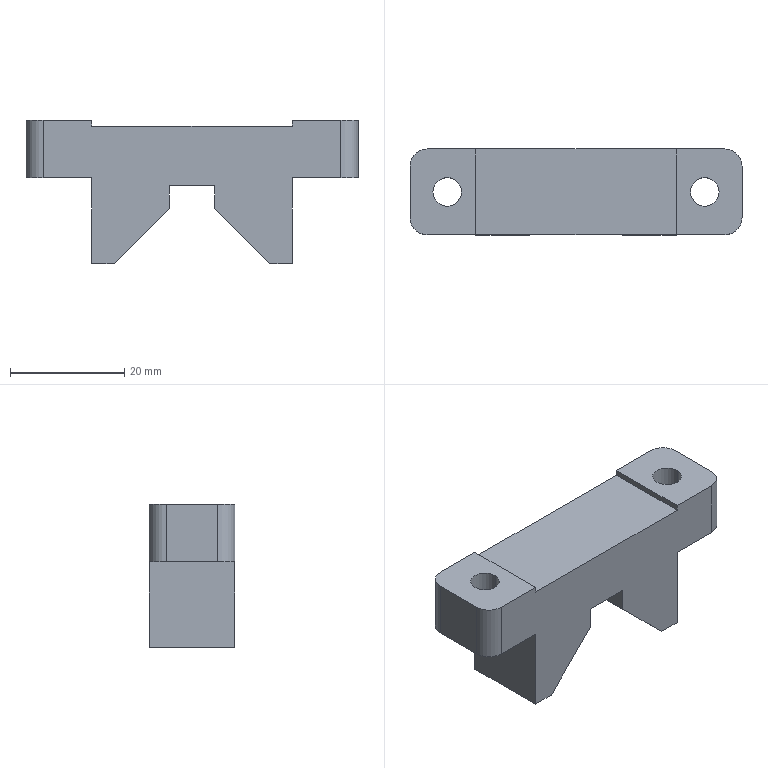Part | SolidWorks | features ICE 2, BaseBody 1, Fillet 1 | 1 solid | 28 faces | box 58 x 15 x 25 mm | volume 12562 mm3 | plane 20 | cylinder 8 | commonest cylinder face diameters 5 x4 6 x4
STEP:
#1=CARTESIAN_POINT('',(60.,7.5,-10.));
#2=VERTEX_POINT('',#1);
#3=CARTESIAN_POINT('',(65.,7.5,-10.));
#4=VERTEX_POINT('',#3);
#5=CARTESIAN_POINT('',(62.5,7.5,-10.));
#6=DIRECTION('',(0.,0.,1.));
#7=DIRECTION('',(1.,0.,0.));
#8=AXIS2_PLACEMENT_3D('',#5,#6,#7);
#9=CIRCLE('',#8,2.5);
#10=EDGE_CURVE('',#2,#4,#9,.T.);
#11=ORIENTED_EDGE('',*,*,#10,.F.);
#12=CARTESIAN_POINT('',(60.,7.5,0.));
#13=VERTEX_POINT('',#12);
#14=CARTESIAN_POINT('',(60.,7.5,-10.));
#15=DIRECTION('',(0.,0.,1.));
#16=VECTOR('',#15,1000.);
#17=LINE('',#14,#16);
#18=EDGE_CURVE('',#2,#13,#17,.T.);
#19=ORIENTED_EDGE('',*,*,#18,.T.);
#20=CARTESIAN_POINT('',(65.,7.5,0.));
#21=VERTEX_POINT('',#20);
#22=CARTESIAN_POINT('',(62.5,7.5,0.));
#23=DIRECTION('',(0.,0.,1.));
#24=DIRECTION('',(1.,0.,0.));
#25=AXIS2_PLACEMENT_3D('',#22,#23,#24);
#26=CIRCLE('',#25,2.5);
#27=EDGE_CURVE('',#13,#21,#26,.T.);
#28=ORIENTED_EDGE('',*,*,#27,.T.);
#29=CARTESIAN_POINT('',(65.,7.5,-10.));
#30=DIRECTION('',(0.,0.,1.));
#31=VECTOR('',#30,1000.);
#32=LINE('',#29,#31);
#33=EDGE_CURVE('',#4,#21,#32,.T.);
#34=ORIENTED_EDGE('',*,*,#33,.F.);
#35=EDGE_LOOP('',(#11,#19,#28,#34));
#36=FACE_OUTER_BOUND('',#35,.T.);
#37=CARTESIAN_POINT('',(62.5,7.5,-10.));
#38=DIRECTION('',(0.,0.,1.));
#39=DIRECTION('',(1.,0.,0.));
#40=AXIS2_PLACEMENT_3D('',#37,#38,#39);
#41=CYLINDRICAL_SURFACE('',#40,2.5);
#42=ADVANCED_FACE('',(#36),#41,.F.);
#43=CARTESIAN_POINT('',(20.,7.5,-10.));
#44=VERTEX_POINT('',#43);
#45=CARTESIAN_POINT('',(15.,7.5,-10.));
#46=VERTEX_POINT('',#45);
#47=CARTESIAN_POINT('',(17.5,7.5,-10.));
#48=DIRECTION('',(0.,0.,-1.));
#49=DIRECTION('',(1.,0.,0.));
#50=AXIS2_PLACEMENT_3D('',#47,#48,#49);
#51=CIRCLE('',#50,2.5);
#52=EDGE_CURVE('',#44,#46,#51,.T.);
#53=ORIENTED_EDGE('',*,*,#52,.T.);
#54=CARTESIAN_POINT('',(15.,7.5,0.));
#55=VERTEX_POINT('',#54);
#56=CARTESIAN_POINT('',(15.,7.5,-10.));
#57=DIRECTION('',(0.,0.,1.));
#58=VECTOR('',#57,1000.);
#59=LINE('',#56,#58);
#60=EDGE_CURVE('',#46,#55,#59,.T.);
#61=ORIENTED_EDGE('',*,*,#60,.T.);
#62=CARTESIAN_POINT('',(20.,7.5,0.));
#63=VERTEX_POINT('',#62);
#64=CARTESIAN_POINT('',(17.5,7.5,0.));
#65=DIRECTION('',(0.,0.,1.));
#66=DIRECTION('',(1.,0.,0.));
#67=AXIS2_PLACEMENT_3D('',#64,#65,#66);
#68=CIRCLE('',#67,2.5);
#69=EDGE_CURVE('',#55,#63,#68,.T.);
#70=ORIENTED_EDGE('',*,*,#69,.T.);
#71=CARTESIAN_POINT('',(20.,7.5,-10.));
#72=DIRECTION('',(0.,0.,1.));
#73=VECTOR('',#72,1000.);
#74=LINE('',#71,#73);
#75=EDGE_CURVE('',#44,#63,#74,.T.);
#76=ORIENTED_EDGE('',*,*,#75,.F.);
#77=EDGE_LOOP('',(#53,#61,#70,#76));
#78=FACE_OUTER_BOUND('',#77,.T.);
#79=CARTESIAN_POINT('',(17.5,7.5,-10.));
#80=DIRECTION('',(0.,0.,1.));
#81=DIRECTION('',(1.,0.,0.));
#82=AXIS2_PLACEMENT_3D('',#79,#80,#81);
#83=CYLINDRICAL_SURFACE('',#82,2.5);
#84=ADVANCED_FACE('',(#78),#83,.F.);
#85=CARTESIAN_POINT('',(62.5,7.5,0.));
#86=DIRECTION('',(0.,0.,1.));
#87=DIRECTION('',(1.,0.,0.));
#88=AXIS2_PLACEMENT_3D('',#85,#86,#87);
#89=CIRCLE('',#88,2.5);
#90=EDGE_CURVE('',#21,#13,#89,.T.);
#91=ORIENTED_EDGE('',*,*,#90,.F.);
#92=ORIENTED_EDGE('',*,*,#27,.F.);
#93=EDGE_LOOP('',(#91,#92));
#94=FACE_BOUND('',#93,.T.);
#95=CARTESIAN_POINT('',(57.5,15.,0.));
#96=VERTEX_POINT('',#95);
#97=CARTESIAN_POINT('',(66.,15.,0.));
#98=VERTEX_POINT('',#97);
#99=CARTESIAN_POINT('',(0.,15.,0.));
#100=DIRECTION('',(1.,0.,0.));
#101=VECTOR('',#100,1000.);
#102=LINE('',#99,#101);
#103=EDGE_CURVE('',#96,#98,#102,.T.);
#104=ORIENTED_EDGE('',*,*,#103,.F.);
#105=CARTESIAN_POINT('',(57.5,0.,0.));
#106=VERTEX_POINT('',#105);
#107=CARTESIAN_POINT('',(57.5,15.,0.));
#108=DIRECTION('',(0.,-1.,0.));
#109=VECTOR('',#108,1000.);
#110=LINE('',#107,#109);
#111=EDGE_CURVE('',#96,#106,#110,.T.);
#112=ORIENTED_EDGE('',*,*,#111,.T.);
#113=CARTESIAN_POINT('',(66.,0.,0.));
#114=VERTEX_POINT('',#113);
#115=CARTESIAN_POINT('',(0.,0.,0.));
#116=DIRECTION('',(-1.,0.,0.));
#117=VECTOR('',#116,1000.);
#118=LINE('',#115,#117);
#119=EDGE_CURVE('',#114,#106,#118,.T.);
#120=ORIENTED_EDGE('',*,*,#119,.F.);
#121=CARTESIAN_POINT('',(69.,3.,0.));
#122=VERTEX_POINT('',#121);
#123=CARTESIAN_POINT('',(66.,3.,0.));
#124=DIRECTION('',(0.,0.,1.));
#125=DIRECTION('',(-1.,0.,0.));
#126=AXIS2_PLACEMENT_3D('',#123,#124,#125);
#127=CIRCLE('',#126,3.);
#128=EDGE_CURVE('',#114,#122,#127,.T.);
#129=ORIENTED_EDGE('',*,*,#128,.T.);
#130=CARTESIAN_POINT('',(69.,12.,0.));
#131=VERTEX_POINT('',#130);
#132=CARTESIAN_POINT('',(69.,15.,0.));
#133=DIRECTION('',(0.,1.,0.));
#134=VECTOR('',#133,1000.);
#135=LINE('',#132,#134);
#136=EDGE_CURVE('',#122,#131,#135,.T.);
#137=ORIENTED_EDGE('',*,*,#136,.T.);
#138=CARTESIAN_POINT('',(66.,12.,0.));
#139=DIRECTION('',(0.,0.,1.));
#140=DIRECTION('',(-1.,0.,0.));
#141=AXIS2_PLACEMENT_3D('',#138,#139,#140);
#142=CIRCLE('',#141,3.);
#143=EDGE_CURVE('',#131,#98,#142,.T.);
#144=ORIENTED_EDGE('',*,*,#143,.T.);
#145=EDGE_LOOP('',(#104,#112,#120,#129,#137,#144));
#146=FACE_OUTER_BOUND('',#145,.T.);
#147=CARTESIAN_POINT('',(0.,15.,0.));
#148=DIRECTION('',(0.,0.,-1.));
#149=DIRECTION('',(-1.,0.,0.));
#150=AXIS2_PLACEMENT_3D('',#147,#148,#149);
#151=PLANE('',#150);
#152=ADVANCED_FACE('',(#94,#146),#151,.F.);
#153=CARTESIAN_POINT('',(57.5,15.,-1.));
#154=VERTEX_POINT('',#153);
#155=CARTESIAN_POINT('',(57.5,15.,0.));
#156=DIRECTION('',(0.,0.,1.));
#157=VECTOR('',#156,1000.);
#158=LINE('',#155,#157);
#159=EDGE_CURVE('',#154,#96,#158,.T.);
#160=ORIENTED_EDGE('',*,*,#159,.T.);
#161=ORIENTED_EDGE('',*,*,#103,.T.);
#162=CARTESIAN_POINT('',(66.,15.,-10.));
#163=VERTEX_POINT('',#162);
#164=CARTESIAN_POINT('',(66.,15.,-10.));
#165=DIRECTION('',(0.,0.,-1.));
#166=VECTOR('',#165,1000.);
#167=LINE('',#164,#166);
#168=EDGE_CURVE('',#98,#163,#167,.T.);
#169=ORIENTED_EDGE('',*,*,#168,.T.);
#170=CARTESIAN_POINT('',(57.5,15.,-10.));
#171=VERTEX_POINT('',#170);
#172=CARTESIAN_POINT('',(0.,15.,-10.));
#173=DIRECTION('',(-1.,0.,0.));
#174=VECTOR('',#173,1000.);
#175=LINE('',#172,#174);
#176=EDGE_CURVE('',#163,#171,#175,.T.);
#177=ORIENTED_EDGE('',*,*,#176,.T.);
#178=CARTESIAN_POINT('',(57.5,15.,-25.));
#179=VERTEX_POINT('',#178);
#180=CARTESIAN_POINT('',(57.5,15.,0.));
#181=DIRECTION('',(0.,0.,-1.));
#182=VECTOR('',#181,1000.);
#183=LINE('',#180,#182);
#184=EDGE_CURVE('',#171,#179,#183,.T.);
#185=ORIENTED_EDGE('',*,*,#184,.T.);
#186=CARTESIAN_POINT('',(53.61,15.,-25.));
#187=VERTEX_POINT('',#186);
#188=CARTESIAN_POINT('',(0.,15.,-25.));
#189=DIRECTION('',(-1.,0.,0.));
#190=VECTOR('',#189,1000.);
#191=LINE('',#188,#190);
#192=EDGE_CURVE('',#179,#187,#191,.T.);
#193=ORIENTED_EDGE('',*,*,#192,.T.);
#194=CARTESIAN_POINT('',(44.,15.,-15.39));
#195=VERTEX_POINT('',#194);
#196=CARTESIAN_POINT('',(53.61,15.,-25.));
#197=DIRECTION('',(-0.7071,0.,0.7071));
#198=VECTOR('',#197,1000.);
#199=LINE('',#196,#198);
#200=EDGE_CURVE('',#187,#195,#199,.T.);
#201=ORIENTED_EDGE('',*,*,#200,.T.);
#202=CARTESIAN_POINT('',(44.,15.,-11.39));
#203=VERTEX_POINT('',#202);
#204=CARTESIAN_POINT('',(44.,15.,0.));
#205=DIRECTION('',(0.,0.,1.));
#206=VECTOR('',#205,1000.);
#207=LINE('',#204,#206);
#208=EDGE_CURVE('',#195,#203,#207,.T.);
#209=ORIENTED_EDGE('',*,*,#208,.T.);
#210=CARTESIAN_POINT('',(36.,15.,-11.39));
#211=VERTEX_POINT('',#210);
#212=CARTESIAN_POINT('',(0.,15.,-11.39));
#213=DIRECTION('',(-1.,0.,0.));
#214=VECTOR('',#213,1000.);
#215=LINE('',#212,#214);
#216=EDGE_CURVE('',#203,#211,#215,.T.);
#217=ORIENTED_EDGE('',*,*,#216,.T.);
#218=CARTESIAN_POINT('',(36.,15.,-15.39));
#219=VERTEX_POINT('',#218);
#220=CARTESIAN_POINT('',(36.,15.,0.));
#221=DIRECTION('',(0.,0.,-1.));
#222=VECTOR('',#221,1000.);
#223=LINE('',#220,#222);
#224=EDGE_CURVE('',#211,#219,#223,.T.);
#225=ORIENTED_EDGE('',*,*,#224,.T.);
#226=CARTESIAN_POINT('',(26.39,15.,-25.));
#227=VERTEX_POINT('',#226);
#228=CARTESIAN_POINT('',(36.,15.,-15.39));
#229=DIRECTION('',(-0.7071,0.,-0.7071));
#230=VECTOR('',#229,1000.);
#231=LINE('',#228,#230);
#232=EDGE_CURVE('',#219,#227,#231,.T.);
#233=ORIENTED_EDGE('',*,*,#232,.T.);
#234=CARTESIAN_POINT('',(22.5,15.,-25.));
#235=VERTEX_POINT('',#234);
#236=CARTESIAN_POINT('',(0.,15.,-25.));
#237=DIRECTION('',(-1.,0.,0.));
#238=VECTOR('',#237,1000.);
#239=LINE('',#236,#238);
#240=EDGE_CURVE('',#227,#235,#239,.T.);
#241=ORIENTED_EDGE('',*,*,#240,.T.);
#242=CARTESIAN_POINT('',(22.5,15.,-10.));
#243=VERTEX_POINT('',#242);
#244=CARTESIAN_POINT('',(22.5,15.,0.));
#245=DIRECTION('',(0.,0.,1.));
#246=VECTOR('',#245,1000.);
#247=LINE('',#244,#246);
#248=EDGE_CURVE('',#235,#243,#247,.T.);
#249=ORIENTED_EDGE('',*,*,#248,.T.);
#250=CARTESIAN_POINT('',(14.,15.,-10.));
#251=VERTEX_POINT('',#250);
#252=CARTESIAN_POINT('',(0.,15.,-10.));
#253=DIRECTION('',(-1.,0.,0.));
#254=VECTOR('',#253,1000.);
#255=LINE('',#252,#254);
#256=EDGE_CURVE('',#243,#251,#255,.T.);
#257=ORIENTED_EDGE('',*,*,#256,.T.);
#258=CARTESIAN_POINT('',(14.,15.,0.));
#259=VERTEX_POINT('',#258);
#260=CARTESIAN_POINT('',(14.,15.,0.));
#261=DIRECTION('',(0.,0.,1.));
#262=VECTOR('',#261,1000.);
#263=LINE('',#260,#262);
#264=EDGE_CURVE('',#251,#259,#263,.T.);
#265=ORIENTED_EDGE('',*,*,#264,.T.);
#266=CARTESIAN_POINT('',(22.5,15.,0.));
#267=VERTEX_POINT('',#266);
#268=CARTESIAN_POINT('',(0.,15.,0.));
#269=DIRECTION('',(1.,0.,0.));
#270=VECTOR('',#269,1000.);
#271=LINE('',#268,#270);
#272=EDGE_CURVE('',#259,#267,#271,.T.);
#273=ORIENTED_EDGE('',*,*,#272,.T.);
#274=CARTESIAN_POINT('',(22.5,15.,-1.));
#275=VERTEX_POINT('',#274);
#276=CARTESIAN_POINT('',(22.5,15.,0.));
#277=DIRECTION('',(0.,0.,-1.));
#278=VECTOR('',#277,1000.);
#279=LINE('',#276,#278);
#280=EDGE_CURVE('',#267,#275,#279,.T.);
#281=ORIENTED_EDGE('',*,*,#280,.T.);
#282=CARTESIAN_POINT('',(57.5,15.,-1.));
#283=DIRECTION('',(1.,0.,0.));
#284=VECTOR('',#283,1000.);
#285=LINE('',#282,#284);
#286=EDGE_CURVE('',#275,#154,#285,.T.);
#287=ORIENTED_EDGE('',*,*,#286,.T.);
#288=EDGE_LOOP('',(#160,#161,#169,#177,#185,#193,#201,#209,#217,#225,#233,#241,#249,#257,#265,#273,#281,#287));
#289=FACE_OUTER_BOUND('',#288,.T.);
#290=CARTESIAN_POINT('',(0.,15.,0.));
#291=DIRECTION('',(0.,1.,0.));
#292=DIRECTION('',(0.,0.,1.));
#293=AXIS2_PLACEMENT_3D('',#290,#291,#292);
#294=PLANE('',#293);
#295=ADVANCED_FACE('',(#289),#294,.T.);
#296=CARTESIAN_POINT('',(36.,0.,-11.39));
#297=VERTEX_POINT('',#296);
#298=CARTESIAN_POINT('',(36.,16.5,-11.39));
#299=DIRECTION('',(0.,1.,0.));
#300=VECTOR('',#299,1000.);
#301=LINE('',#298,#300);
#302=EDGE_CURVE('',#297,#211,#301,.T.);
#303=ORIENTED_EDGE('',*,*,#302,.F.);
#304=CARTESIAN_POINT('',(36.,0.,-15.39));
#305=VERTEX_POINT('',#304);
#306=CARTESIAN_POINT('',(36.,0.,-11.39));
#307=DIRECTION('',(0.,0.,1.));
#308=VECTOR('',#307,1000.);
#309=LINE('',#306,#308);
#310=EDGE_CURVE('',#305,#297,#309,.T.);
#311=ORIENTED_EDGE('',*,*,#310,.F.);
#312=CARTESIAN_POINT('',(36.,16.5,-15.39));
#313=DIRECTION('',(0.,-1.,0.));
#314=VECTOR('',#313,1000.);
#315=LINE('',#312,#314);
#316=EDGE_CURVE('',#219,#305,#315,.T.);
#317=ORIENTED_EDGE('',*,*,#316,.F.);
#318=ORIENTED_EDGE('',*,*,#224,.F.);
#319=EDGE_LOOP('',(#303,#311,#317,#318));
#320=FACE_OUTER_BOUND('',#319,.T.);
#321=CARTESIAN_POINT('',(36.,16.5,-11.39));
#322=DIRECTION('',(-1.,0.,0.));
#323=DIRECTION('',(0.,0.,1.));
#324=AXIS2_PLACEMENT_3D('',#321,#322,#323);
#325=PLANE('',#324);
#326=ADVANCED_FACE('',(#320),#325,.F.);
#327=CARTESIAN_POINT('',(44.,0.,-11.39));
#328=VERTEX_POINT('',#327);
#329=CARTESIAN_POINT('',(44.,16.5,-11.39));
#330=DIRECTION('',(0.,1.,0.));
#331=VECTOR('',#330,1000.);
#332=LINE('',#329,#331);
#333=EDGE_CURVE('',#328,#203,#332,.T.);
#334=ORIENTED_EDGE('',*,*,#333,.F.);
#335=CARTESIAN_POINT('',(44.,0.,-11.39));
#336=DIRECTION('',(1.,0.,0.));
#337=VECTOR('',#336,1000.);
#338=LINE('',#335,#337);
#339=EDGE_CURVE('',#297,#328,#338,.T.);
#340=ORIENTED_EDGE('',*,*,#339,.F.);
#341=ORIENTED_EDGE('',*,*,#302,.T.);
#342=ORIENTED_EDGE('',*,*,#216,.F.);
#343=EDGE_LOOP('',(#334,#340,#341,#342));
#344=FACE_OUTER_BOUND('',#343,.T.);
#345=CARTESIAN_POINT('',(44.,16.5,-11.39));
#346=DIRECTION('',(0.,0.,1.));
#347=DIRECTION('',(1.,0.,0.));
#348=AXIS2_PLACEMENT_3D('',#345,#346,#347);
#349=PLANE('',#348);
#350=ADVANCED_FACE('',(#344),#349,.F.);
#351=CARTESIAN_POINT('',(44.,0.,-15.39));
#352=VERTEX_POINT('',#351);
#353=CARTESIAN_POINT('',(44.,16.5,-15.39));
#354=DIRECTION('',(0.,1.,0.));
#355=VECTOR('',#354,1000.);
#356=LINE('',#353,#355);
#357=EDGE_CURVE('',#352,#195,#356,.T.);
#358=ORIENTED_EDGE('',*,*,#357,.F.);
#359=CARTESIAN_POINT('',(44.,0.,-15.39));
#360=DIRECTION('',(0.,0.,-1.));
#361=VECTOR('',#360,1000.);
#362=LINE('',#359,#361);
#363=EDGE_CURVE('',#328,#352,#362,.T.);
#364=ORIENTED_EDGE('',*,*,#363,.F.);
#365=ORIENTED_EDGE('',*,*,#333,.T.);
#366=ORIENTED_EDGE('',*,*,#208,.F.);
#367=EDGE_LOOP('',(#358,#364,#365,#366));
#368=FACE_OUTER_BOUND('',#367,.T.);
#369=CARTESIAN_POINT('',(44.,16.5,-15.39));
#370=DIRECTION('',(1.,0.,0.));
#371=DIRECTION('',(0.,0.,-1.));
#372=AXIS2_PLACEMENT_3D('',#369,#370,#371);
#373=PLANE('',#372);
#374=ADVANCED_FACE('',(#368),#373,.F.);
#375=CARTESIAN_POINT('',(53.61,0.,-25.));
#376=VERTEX_POINT('',#375);
#377=CARTESIAN_POINT('',(53.61,16.5,-25.));
#378=DIRECTION('',(0.,1.,0.));
#379=VECTOR('',#378,1000.);
#380=LINE('',#377,#379);
#381=EDGE_CURVE('',#376,#187,#380,.T.);
#382=ORIENTED_EDGE('',*,*,#381,.F.);
#383=CARTESIAN_POINT('',(53.61,0.,-25.));
#384=DIRECTION('',(0.7071,0.,-0.7071));
#385=VECTOR('',#384,1000.);
#386=LINE('',#383,#385);
#387=EDGE_CURVE('',#352,#376,#386,.T.);
#388=ORIENTED_EDGE('',*,*,#387,.F.);
#389=ORIENTED_EDGE('',*,*,#357,.T.);
#390=ORIENTED_EDGE('',*,*,#200,.F.);
#391=EDGE_LOOP('',(#382,#388,#389,#390));
#392=FACE_OUTER_BOUND('',#391,.T.);
#393=CARTESIAN_POINT('',(53.61,16.5,-25.));
#394=DIRECTION('',(0.7071,0.,0.7071));
#395=DIRECTION('',(0.7071,0.,-0.7071));
#396=AXIS2_PLACEMENT_3D('',#393,#394,#395);
#397=PLANE('',#396);
#398=ADVANCED_FACE('',(#392),#397,.F.);
#399=ORIENTED_EDGE('',*,*,#192,.F.);
#400=CARTESIAN_POINT('',(57.5,0.,-25.));
#401=VERTEX_POINT('',#400);
#402=CARTESIAN_POINT('',(57.5,15.,-25.));
#403=DIRECTION('',(0.,1.,0.));
#404=VECTOR('',#403,1000.);
#405=LINE('',#402,#404);
#406=EDGE_CURVE('',#401,#179,#405,.T.);
#407=ORIENTED_EDGE('',*,*,#406,.F.);
#408=CARTESIAN_POINT('',(80.,0.,-25.));
#409=DIRECTION('',(1.,0.,0.));
#410=VECTOR('',#409,1000.);
#411=LINE('',#408,#410);
#412=EDGE_CURVE('',#376,#401,#411,.T.);
#413=ORIENTED_EDGE('',*,*,#412,.F.);
#414=ORIENTED_EDGE('',*,*,#381,.T.);
#415=EDGE_LOOP('',(#399,#407,#413,#414));
#416=FACE_OUTER_BOUND('',#415,.T.);
#417=CARTESIAN_POINT('',(80.,15.,-25.));
#418=DIRECTION('',(0.,0.,1.));
#419=DIRECTION('',(1.,0.,0.));
#420=AXIS2_PLACEMENT_3D('',#417,#418,#419);
#421=PLANE('',#420);
#422=ADVANCED_FACE('',(#416),#421,.F.);
#423=ORIENTED_EDGE('',*,*,#406,.T.);
#424=ORIENTED_EDGE('',*,*,#184,.F.);
#425=CARTESIAN_POINT('',(57.5,0.,-10.));
#426=VERTEX_POINT('',#425);
#427=CARTESIAN_POINT('',(57.5,16.5,-10.));
#428=DIRECTION('',(0.,-1.,0.));
#429=VECTOR('',#428,1000.);
#430=LINE('',#427,#429);
#431=EDGE_CURVE('',#171,#426,#430,.T.);
#432=ORIENTED_EDGE('',*,*,#431,.T.);
#433=CARTESIAN_POINT('',(57.5,0.,-25.));
#434=DIRECTION('',(0.,0.,-1.));
#435=VECTOR('',#434,1000.);
#436=LINE('',#433,#435);
#437=EDGE_CURVE('',#426,#401,#436,.T.);
#438=ORIENTED_EDGE('',*,*,#437,.T.);
#439=EDGE_LOOP('',(#423,#424,#432,#438));
#440=FACE_OUTER_BOUND('',#439,.T.);
#441=CARTESIAN_POINT('',(57.5,16.5,-25.));
#442=DIRECTION('',(1.,0.,0.));
#443=DIRECTION('',(0.,0.,-1.));
#444=AXIS2_PLACEMENT_3D('',#441,#442,#443);
#445=PLANE('',#444);
#446=ADVANCED_FACE('',(#440),#445,.T.);
#447=ORIENTED_EDGE('',*,*,#176,.F.);
#448=CARTESIAN_POINT('',(69.,12.,-10.));
#449=VERTEX_POINT('',#448);
#450=CARTESIAN_POINT('',(66.,12.,-10.));
#451=DIRECTION('',(0.,0.,-1.));
#452=DIRECTION('',(-1.,0.,0.));
#453=AXIS2_PLACEMENT_3D('',#450,#451,#452);
#454=CIRCLE('',#453,3.);
#455=EDGE_CURVE('',#163,#449,#454,.T.);
#456=ORIENTED_EDGE('',*,*,#455,.T.);
#457=CARTESIAN_POINT('',(69.,3.,-10.));
#458=VERTEX_POINT('',#457);
#459=CARTESIAN_POINT('',(69.,15.,-10.));
#460=DIRECTION('',(0.,1.,0.));
#461=VECTOR('',#460,1000.);
#462=LINE('',#459,#461);
#463=EDGE_CURVE('',#458,#449,#462,.T.);
#464=ORIENTED_EDGE('',*,*,#463,.F.);
#465=CARTESIAN_POINT('',(66.,0.,-10.));
#466=VERTEX_POINT('',#465);
#467=CARTESIAN_POINT('',(66.,3.,-10.));
#468=DIRECTION('',(0.,0.,-1.));
#469=DIRECTION('',(-1.,0.,0.));
#470=AXIS2_PLACEMENT_3D('',#467,#468,#469);
#471=CIRCLE('',#470,3.);
#472=EDGE_CURVE('',#458,#466,#471,.T.);
#473=ORIENTED_EDGE('',*,*,#472,.T.);
#474=CARTESIAN_POINT('',(57.5,0.,-10.));
#475=DIRECTION('',(-1.,0.,0.));
#476=VECTOR('',#475,1000.);
#477=LINE('',#474,#476);
#478=EDGE_CURVE('',#466,#426,#477,.T.);
#479=ORIENTED_EDGE('',*,*,#478,.T.);
#480=ORIENTED_EDGE('',*,*,#431,.F.);
#481=EDGE_LOOP('',(#447,#456,#464,#473,#479,#480));
#482=FACE_OUTER_BOUND('',#481,.T.);
#483=CARTESIAN_POINT('',(62.5,7.5,-10.));
#484=DIRECTION('',(0.,0.,1.));
#485=DIRECTION('',(1.,0.,0.));
#486=AXIS2_PLACEMENT_3D('',#483,#484,#485);
#487=CIRCLE('',#486,2.5);
#488=EDGE_CURVE('',#4,#2,#487,.T.);
#489=ORIENTED_EDGE('',*,*,#488,.T.);
#490=ORIENTED_EDGE('',*,*,#10,.T.);
#491=EDGE_LOOP('',(#489,#490));
#492=FACE_BOUND('',#491,.T.);
#493=CARTESIAN_POINT('',(57.5,16.5,-10.));
#494=DIRECTION('',(0.,0.,-1.));
#495=DIRECTION('',(-1.,0.,0.));
#496=AXIS2_PLACEMENT_3D('',#493,#494,#495);
#497=PLANE('',#496);
#498=ADVANCED_FACE('',(#482,#492),#497,.T.);
#499=CARTESIAN_POINT('',(22.5,0.,0.));
#500=VERTEX_POINT('',#499);
#501=CARTESIAN_POINT('',(14.,0.,0.));
#502=VERTEX_POINT('',#501);
#503=CARTESIAN_POINT('',(0.,0.,0.));
#504=DIRECTION('',(-1.,0.,0.));
#505=VECTOR('',#504,1000.);
#506=LINE('',#503,#505);
#507=EDGE_CURVE('',#500,#502,#506,.T.);
#508=ORIENTED_EDGE('',*,*,#507,.F.);
#509=CARTESIAN_POINT('',(22.5,15.,0.));
#510=DIRECTION('',(0.,-1.,0.));
#511=VECTOR('',#510,1000.);
#512=LINE('',#509,#511);
#513=EDGE_CURVE('',#267,#500,#512,.T.);
#514=ORIENTED_EDGE('',*,*,#513,.F.);
#515=ORIENTED_EDGE('',*,*,#272,.F.);
#516=CARTESIAN_POINT('',(11.,12.,0.));
#517=VERTEX_POINT('',#516);
#518=CARTESIAN_POINT('',(14.,12.,0.));
#519=DIRECTION('',(0.,0.,1.));
#520=DIRECTION('',(-1.,0.,0.));
#521=AXIS2_PLACEMENT_3D('',#518,#519,#520);
#522=CIRCLE('',#521,3.);
#523=EDGE_CURVE('',#259,#517,#522,.T.);
#524=ORIENTED_EDGE('',*,*,#523,.T.);
#525=CARTESIAN_POINT('',(11.,3.,0.));
#526=VERTEX_POINT('',#525);
#527=CARTESIAN_POINT('',(11.,15.,0.));
#528=DIRECTION('',(0.,-1.,0.));
#529=VECTOR('',#528,1000.);
#530=LINE('',#527,#529);
#531=EDGE_CURVE('',#517,#526,#530,.T.);
#532=ORIENTED_EDGE('',*,*,#531,.T.);
#533=CARTESIAN_POINT('',(14.,3.,0.));
#534=DIRECTION('',(0.,0.,1.));
#535=DIRECTION('',(-1.,0.,0.));
#536=AXIS2_PLACEMENT_3D('',#533,#534,#535);
#537=CIRCLE('',#536,3.);
#538=EDGE_CURVE('',#526,#502,#537,.T.);
#539=ORIENTED_EDGE('',*,*,#538,.T.);
#540=EDGE_LOOP('',(#508,#514,#515,#524,#532,#539));
#541=FACE_OUTER_BOUND('',#540,.T.);
#542=CARTESIAN_POINT('',(17.5,7.5,0.));
#543=DIRECTION('',(0.,0.,1.));
#544=DIRECTION('',(1.,0.,0.));
#545=AXIS2_PLACEMENT_3D('',#542,#543,#544);
#546=CIRCLE('',#545,2.5);
#547=EDGE_CURVE('',#63,#55,#546,.T.);
#548=ORIENTED_EDGE('',*,*,#547,.F.);
#549=ORIENTED_EDGE('',*,*,#69,.F.);
#550=EDGE_LOOP('',(#548,#549));
#551=FACE_BOUND('',#550,.T.);
#552=CARTESIAN_POINT('',(0.,15.,0.));
#553=DIRECTION('',(0.,0.,-1.));
#554=DIRECTION('',(-1.,0.,0.));
#555=AXIS2_PLACEMENT_3D('',#552,#553,#554);
#556=PLANE('',#555);
#557=ADVANCED_FACE('',(#541,#551),#556,.F.);
#558=CARTESIAN_POINT('',(11.,12.,-10.));
#559=VERTEX_POINT('',#558);
#560=CARTESIAN_POINT('',(11.,3.,-10.));
#561=VERTEX_POINT('',#560);
#562=CARTESIAN_POINT('',(11.,15.,-10.));
#563=DIRECTION('',(0.,-1.,0.));
#564=VECTOR('',#563,1000.);
#565=LINE('',#562,#564);
#566=EDGE_CURVE('',#559,#561,#565,.T.);
#567=ORIENTED_EDGE('',*,*,#566,.F.);
#568=CARTESIAN_POINT('',(14.,12.,-10.));
#569=DIRECTION('',(0.,0.,-1.));
#570=DIRECTION('',(1.,0.,0.));
#571=AXIS2_PLACEMENT_3D('',#568,#569,#570);
#572=CIRCLE('',#571,3.);
#573=EDGE_CURVE('',#559,#251,#572,.T.);
#574=ORIENTED_EDGE('',*,*,#573,.T.);
#575=ORIENTED_EDGE('',*,*,#256,.F.);
#576=CARTESIAN_POINT('',(22.5,0.,-10.));
#577=VERTEX_POINT('',#576);
#578=CARTESIAN_POINT('',(22.5,16.5,-10.));
#579=DIRECTION('',(0.,1.,0.));
#580=VECTOR('',#579,1000.);
#581=LINE('',#578,#580);
#582=EDGE_CURVE('',#577,#243,#581,.T.);
#583=ORIENTED_EDGE('',*,*,#582,.F.);
#584=CARTESIAN_POINT('',(14.,0.,-10.));
#585=VERTEX_POINT('',#584);
#586=CARTESIAN_POINT('',(22.5,0.,-10.));
#587=DIRECTION('',(1.,0.,0.));
#588=VECTOR('',#587,1000.);
#589=LINE('',#586,#588);
#590=EDGE_CURVE('',#585,#577,#589,.T.);
#591=ORIENTED_EDGE('',*,*,#590,.F.);
#592=CARTESIAN_POINT('',(14.,3.,-10.));
#593=DIRECTION('',(0.,0.,-1.));
#594=DIRECTION('',(1.,0.,0.));
#595=AXIS2_PLACEMENT_3D('',#592,#593,#594);
#596=CIRCLE('',#595,3.);
#597=EDGE_CURVE('',#585,#561,#596,.T.);
#598=ORIENTED_EDGE('',*,*,#597,.T.);
#599=EDGE_LOOP('',(#567,#574,#575,#583,#591,#598));
#600=FACE_OUTER_BOUND('',#599,.T.);
#601=ORIENTED_EDGE('',*,*,#52,.F.);
#602=CARTESIAN_POINT('',(17.5,7.5,-10.));
#603=DIRECTION('',(0.,0.,-1.));
#604=DIRECTION('',(1.,0.,0.));
#605=AXIS2_PLACEMENT_3D('',#602,#603,#604);
#606=CIRCLE('',#605,2.5);
#607=EDGE_CURVE('',#46,#44,#606,.T.);
#608=ORIENTED_EDGE('',*,*,#607,.F.);
#609=EDGE_LOOP('',(#601,#608));
#610=FACE_BOUND('',#609,.T.);
#611=CARTESIAN_POINT('',(22.5,16.5,-10.));
#612=DIRECTION('',(0.,0.,1.));
#613=DIRECTION('',(1.,0.,0.));
#614=AXIS2_PLACEMENT_3D('',#611,#612,#613);
#615=PLANE('',#614);
#616=ADVANCED_FACE('',(#600,#610),#615,.F.);
#617=CARTESIAN_POINT('',(22.5,0.,-25.));
#618=VERTEX_POINT('',#617);
#619=CARTESIAN_POINT('',(22.5,16.5,-25.));
#620=DIRECTION('',(0.,1.,0.));
#621=VECTOR('',#620,1000.);
#622=LINE('',#619,#621);
#623=EDGE_CURVE('',#618,#235,#622,.T.);
#624=ORIENTED_EDGE('',*,*,#623,.F.);
#625=CARTESIAN_POINT('',(22.5,0.,-25.));
#626=DIRECTION('',(0.,0.,-1.));
#627=VECTOR('',#626,1000.);
#628=LINE('',#625,#627);
#629=EDGE_CURVE('',#577,#618,#628,.T.);
#630=ORIENTED_EDGE('',*,*,#629,.F.);
#631=ORIENTED_EDGE('',*,*,#582,.T.);
#632=ORIENTED_EDGE('',*,*,#248,.F.);
#633=EDGE_LOOP('',(#624,#630,#631,#632));
#634=FACE_OUTER_BOUND('',#633,.T.);
#635=CARTESIAN_POINT('',(22.5,16.5,-25.));
#636=DIRECTION('',(1.,0.,0.));
#637=DIRECTION('',(0.,0.,-1.));
#638=AXIS2_PLACEMENT_3D('',#635,#636,#637);
#639=PLANE('',#638);
#640=ADVANCED_FACE('',(#634),#639,.F.);
#641=CARTESIAN_POINT('',(26.39,0.,-25.));
#642=VERTEX_POINT('',#641);
#643=CARTESIAN_POINT('',(26.39,15.,-25.));
#644=DIRECTION('',(0.,1.,0.));
#645=VECTOR('',#644,1000.);
#646=LINE('',#643,#645);
#647=EDGE_CURVE('',#642,#227,#646,.T.);
#648=ORIENTED_EDGE('',*,*,#647,.F.);
#649=CARTESIAN_POINT('',(80.,0.,-25.));
#650=DIRECTION('',(1.,0.,0.));
#651=VECTOR('',#650,1000.);
#652=LINE('',#649,#651);
#653=EDGE_CURVE('',#618,#642,#652,.T.);
#654=ORIENTED_EDGE('',*,*,#653,.F.);
#655=ORIENTED_EDGE('',*,*,#623,.T.);
#656=ORIENTED_EDGE('',*,*,#240,.F.);
#657=EDGE_LOOP('',(#648,#654,#655,#656));
#658=FACE_OUTER_BOUND('',#657,.T.);
#659=CARTESIAN_POINT('',(80.,15.,-25.));
#660=DIRECTION('',(0.,0.,1.));
#661=DIRECTION('',(1.,0.,0.));
#662=AXIS2_PLACEMENT_3D('',#659,#660,#661);
#663=PLANE('',#662);
#664=ADVANCED_FACE('',(#658),#663,.F.);
#665=ORIENTED_EDGE('',*,*,#316,.T.);
#666=CARTESIAN_POINT('',(36.,0.,-15.39));
#667=DIRECTION('',(0.7071,0.,0.7071));
#668=VECTOR('',#667,1000.);
#669=LINE('',#666,#668);
#670=EDGE_CURVE('',#642,#305,#669,.T.);
#671=ORIENTED_EDGE('',*,*,#670,.F.);
#672=ORIENTED_EDGE('',*,*,#647,.T.);
#673=ORIENTED_EDGE('',*,*,#232,.F.);
#674=EDGE_LOOP('',(#665,#671,#672,#673));
#675=FACE_OUTER_BOUND('',#674,.T.);
#676=CARTESIAN_POINT('',(36.,16.5,-15.39));
#677=DIRECTION('',(-0.7071,0.,0.7071));
#678=DIRECTION('',(0.7071,0.,0.7071));
#679=AXIS2_PLACEMENT_3D('',#676,#677,#678);
#680=PLANE('',#679);
#681=ADVANCED_FACE('',(#675),#680,.F.);
#682=ORIENTED_EDGE('',*,*,#119,.T.);
#683=CARTESIAN_POINT('',(57.5,0.,-1.));
#684=VERTEX_POINT('',#683);
#685=CARTESIAN_POINT('',(57.5,0.,0.));
#686=DIRECTION('',(0.,0.,1.));
#687=VECTOR('',#686,1000.);
#688=LINE('',#685,#687);
#689=EDGE_CURVE('',#684,#106,#688,.T.);
#690=ORIENTED_EDGE('',*,*,#689,.F.);
#691=CARTESIAN_POINT('',(22.5,0.,-1.));
#692=VERTEX_POINT('',#691);
#693=CARTESIAN_POINT('',(57.5,0.,-1.));
#694=DIRECTION('',(1.,0.,0.));
#695=VECTOR('',#694,1000.);
#696=LINE('',#693,#695);
#697=EDGE_CURVE('',#692,#684,#696,.T.);
#698=ORIENTED_EDGE('',*,*,#697,.F.);
#699=CARTESIAN_POINT('',(22.5,0.,0.));
#700=DIRECTION('',(0.,0.,-1.));
#701=VECTOR('',#700,1000.);
#702=LINE('',#699,#701);
#703=EDGE_CURVE('',#500,#692,#702,.T.);
#704=ORIENTED_EDGE('',*,*,#703,.F.);
#705=ORIENTED_EDGE('',*,*,#507,.T.);
#706=CARTESIAN_POINT('',(14.,0.,0.));
#707=DIRECTION('',(0.,0.,-1.));
#708=VECTOR('',#707,1000.);
#709=LINE('',#706,#708);
#710=EDGE_CURVE('',#502,#585,#709,.T.);
#711=ORIENTED_EDGE('',*,*,#710,.T.);
#712=ORIENTED_EDGE('',*,*,#590,.T.);
#713=ORIENTED_EDGE('',*,*,#629,.T.);
#714=ORIENTED_EDGE('',*,*,#653,.T.);
#715=ORIENTED_EDGE('',*,*,#670,.T.);
#716=ORIENTED_EDGE('',*,*,#310,.T.);
#717=ORIENTED_EDGE('',*,*,#339,.T.);
#718=ORIENTED_EDGE('',*,*,#363,.T.);
#719=ORIENTED_EDGE('',*,*,#387,.T.);
#720=ORIENTED_EDGE('',*,*,#412,.T.);
#721=ORIENTED_EDGE('',*,*,#437,.F.);
#722=ORIENTED_EDGE('',*,*,#478,.F.);
#723=CARTESIAN_POINT('',(66.,0.,0.));
#724=DIRECTION('',(0.,0.,1.));
#725=VECTOR('',#724,1000.);
#726=LINE('',#723,#725);
#727=EDGE_CURVE('',#466,#114,#726,.T.);
#728=ORIENTED_EDGE('',*,*,#727,.T.);
#729=EDGE_LOOP('',(#682,#690,#698,#704,#705,#711,#712,#713,#714,#715,#716,#717,#718,#719,#720,#721,#722,#728));
#730=FACE_OUTER_BOUND('',#729,.T.);
#731=CARTESIAN_POINT('',(0.,0.,0.));
#732=DIRECTION('',(0.,1.,0.));
#733=DIRECTION('',(0.,0.,1.));
#734=AXIS2_PLACEMENT_3D('',#731,#732,#733);
#735=PLANE('',#734);
#736=ADVANCED_FACE('',(#730),#735,.F.);
#737=ORIENTED_EDGE('',*,*,#18,.F.);
#738=ORIENTED_EDGE('',*,*,#488,.F.);
#739=ORIENTED_EDGE('',*,*,#33,.T.);
#740=ORIENTED_EDGE('',*,*,#90,.T.);
#741=EDGE_LOOP('',(#737,#738,#739,#740));
#742=FACE_OUTER_BOUND('',#741,.T.);
#743=CARTESIAN_POINT('',(62.5,7.5,-10.));
#744=DIRECTION('',(0.,0.,1.));
#745=DIRECTION('',(1.,0.,0.));
#746=AXIS2_PLACEMENT_3D('',#743,#744,#745);
#747=CYLINDRICAL_SURFACE('',#746,2.5);
#748=ADVANCED_FACE('',(#742),#747,.F.);
#749=ORIENTED_EDGE('',*,*,#60,.F.);
#750=ORIENTED_EDGE('',*,*,#607,.T.);
#751=ORIENTED_EDGE('',*,*,#75,.T.);
#752=ORIENTED_EDGE('',*,*,#547,.T.);
#753=EDGE_LOOP('',(#749,#750,#751,#752));
#754=FACE_OUTER_BOUND('',#753,.T.);
#755=CARTESIAN_POINT('',(17.5,7.5,-10.));
#756=DIRECTION('',(0.,0.,1.));
#757=DIRECTION('',(1.,0.,0.));
#758=AXIS2_PLACEMENT_3D('',#755,#756,#757);
#759=CYLINDRICAL_SURFACE('',#758,2.5);
#760=ADVANCED_FACE('',(#754),#759,.F.);
#761=ORIENTED_EDGE('',*,*,#531,.F.);
#762=CARTESIAN_POINT('',(11.,12.,-10.));
#763=DIRECTION('',(0.,0.,-1.));
#764=VECTOR('',#763,1000.);
#765=LINE('',#762,#764);
#766=EDGE_CURVE('',#517,#559,#765,.T.);
#767=ORIENTED_EDGE('',*,*,#766,.T.);
#768=ORIENTED_EDGE('',*,*,#566,.T.);
#769=CARTESIAN_POINT('',(11.,3.,0.));
#770=DIRECTION('',(0.,0.,1.));
#771=VECTOR('',#770,1000.);
#772=LINE('',#769,#771);
#773=EDGE_CURVE('',#561,#526,#772,.T.);
#774=ORIENTED_EDGE('',*,*,#773,.T.);
#775=EDGE_LOOP('',(#761,#767,#768,#774));
#776=FACE_OUTER_BOUND('',#775,.T.);
#777=CARTESIAN_POINT('',(11.,15.,0.));
#778=DIRECTION('',(1.,0.,0.));
#779=DIRECTION('',(0.,0.,-1.));
#780=AXIS2_PLACEMENT_3D('',#777,#778,#779);
#781=PLANE('',#780);
#782=ADVANCED_FACE('',(#776),#781,.F.);
#783=ORIENTED_EDGE('',*,*,#463,.T.);
#784=CARTESIAN_POINT('',(69.,12.,0.));
#785=DIRECTION('',(0.,0.,1.));
#786=VECTOR('',#785,1000.);
#787=LINE('',#784,#786);
#788=EDGE_CURVE('',#449,#131,#787,.T.);
#789=ORIENTED_EDGE('',*,*,#788,.T.);
#790=ORIENTED_EDGE('',*,*,#136,.F.);
#791=CARTESIAN_POINT('',(69.,3.,0.));
#792=DIRECTION('',(0.,0.,-1.));
#793=VECTOR('',#792,1000.);
#794=LINE('',#791,#793);
#795=EDGE_CURVE('',#122,#458,#794,.T.);
#796=ORIENTED_EDGE('',*,*,#795,.T.);
#797=EDGE_LOOP('',(#783,#789,#790,#796));
#798=FACE_OUTER_BOUND('',#797,.T.);
#799=CARTESIAN_POINT('',(69.,15.,0.));
#800=DIRECTION('',(-1.,0.,0.));
#801=DIRECTION('',(0.,0.,1.));
#802=AXIS2_PLACEMENT_3D('',#799,#800,#801);
#803=PLANE('',#802);
#804=ADVANCED_FACE('',(#798),#803,.F.);
#805=ORIENTED_EDGE('',*,*,#523,.F.);
#806=ORIENTED_EDGE('',*,*,#264,.F.);
#807=ORIENTED_EDGE('',*,*,#573,.F.);
#808=ORIENTED_EDGE('',*,*,#766,.F.);
#809=EDGE_LOOP('',(#805,#806,#807,#808));
#810=FACE_OUTER_BOUND('',#809,.T.);
#811=CARTESIAN_POINT('',(14.,12.,0.));
#812=DIRECTION('',(0.,0.,1.));
#813=DIRECTION('',(1.,0.,0.));
#814=AXIS2_PLACEMENT_3D('',#811,#812,#813);
#815=CYLINDRICAL_SURFACE('',#814,3.);
#816=ADVANCED_FACE('',(#810),#815,.T.);
#817=ORIENTED_EDGE('',*,*,#538,.F.);
#818=ORIENTED_EDGE('',*,*,#773,.F.);
#819=ORIENTED_EDGE('',*,*,#597,.F.);
#820=ORIENTED_EDGE('',*,*,#710,.F.);
#821=EDGE_LOOP('',(#817,#818,#819,#820));
#822=FACE_OUTER_BOUND('',#821,.T.);
#823=CARTESIAN_POINT('',(14.,3.,0.));
#824=DIRECTION('',(0.,0.,-1.));
#825=DIRECTION('',(-1.,0.,0.));
#826=AXIS2_PLACEMENT_3D('',#823,#824,#825);
#827=CYLINDRICAL_SURFACE('',#826,3.);
#828=ADVANCED_FACE('',(#822),#827,.T.);
#829=ORIENTED_EDGE('',*,*,#143,.F.);
#830=ORIENTED_EDGE('',*,*,#788,.F.);
#831=ORIENTED_EDGE('',*,*,#455,.F.);
#832=ORIENTED_EDGE('',*,*,#168,.F.);
#833=EDGE_LOOP('',(#829,#830,#831,#832));
#834=FACE_OUTER_BOUND('',#833,.T.);
#835=CARTESIAN_POINT('',(66.,12.,0.));
#836=DIRECTION('',(0.,0.,1.));
#837=DIRECTION('',(1.,0.,0.));
#838=AXIS2_PLACEMENT_3D('',#835,#836,#837);
#839=CYLINDRICAL_SURFACE('',#838,3.);
#840=ADVANCED_FACE('',(#834),#839,.T.);
#841=ORIENTED_EDGE('',*,*,#128,.F.);
#842=ORIENTED_EDGE('',*,*,#727,.F.);
#843=ORIENTED_EDGE('',*,*,#472,.F.);
#844=ORIENTED_EDGE('',*,*,#795,.F.);
#845=EDGE_LOOP('',(#841,#842,#843,#844));
#846=FACE_OUTER_BOUND('',#845,.T.);
#847=CARTESIAN_POINT('',(66.,3.,0.));
#848=DIRECTION('',(0.,0.,-1.));
#849=DIRECTION('',(-1.,0.,0.));
#850=AXIS2_PLACEMENT_3D('',#847,#848,#849);
#851=CYLINDRICAL_SURFACE('',#850,3.);
#852=ADVANCED_FACE('',(#846),#851,.T.);
#853=ORIENTED_EDGE('',*,*,#689,.T.);
#854=ORIENTED_EDGE('',*,*,#111,.F.);
#855=ORIENTED_EDGE('',*,*,#159,.F.);
#856=CARTESIAN_POINT('',(57.5,15.,-1.));
#857=DIRECTION('',(0.,-1.,0.));
#858=VECTOR('',#857,1000.);
#859=LINE('',#856,#858);
#860=EDGE_CURVE('',#154,#684,#859,.T.);
#861=ORIENTED_EDGE('',*,*,#860,.T.);
#862=EDGE_LOOP('',(#853,#854,#855,#861));
#863=FACE_OUTER_BOUND('',#862,.T.);
#864=CARTESIAN_POINT('',(57.5,15.,0.));
#865=DIRECTION('',(1.,0.,0.));
#866=DIRECTION('',(0.,0.,-1.));
#867=AXIS2_PLACEMENT_3D('',#864,#865,#866);
#868=PLANE('',#867);
#869=ADVANCED_FACE('',(#863),#868,.F.);
#870=ORIENTED_EDGE('',*,*,#697,.T.);
#871=ORIENTED_EDGE('',*,*,#860,.F.);
#872=ORIENTED_EDGE('',*,*,#286,.F.);
#873=CARTESIAN_POINT('',(22.5,15.,-1.));
#874=DIRECTION('',(0.,-1.,0.));
#875=VECTOR('',#874,1000.);
#876=LINE('',#873,#875);
#877=EDGE_CURVE('',#275,#692,#876,.T.);
#878=ORIENTED_EDGE('',*,*,#877,.T.);
#879=EDGE_LOOP('',(#870,#871,#872,#878));
#880=FACE_OUTER_BOUND('',#879,.T.);
#881=CARTESIAN_POINT('',(57.5,15.,-1.));
#882=DIRECTION('',(0.,0.,-1.));
#883=DIRECTION('',(-1.,0.,0.));
#884=AXIS2_PLACEMENT_3D('',#881,#882,#883);
#885=PLANE('',#884);
#886=ADVANCED_FACE('',(#880),#885,.F.);
#887=ORIENTED_EDGE('',*,*,#703,.T.);
#888=ORIENTED_EDGE('',*,*,#877,.F.);
#889=ORIENTED_EDGE('',*,*,#280,.F.);
#890=ORIENTED_EDGE('',*,*,#513,.T.);
#891=EDGE_LOOP('',(#887,#888,#889,#890));
#892=FACE_OUTER_BOUND('',#891,.T.);
#893=CARTESIAN_POINT('',(22.5,15.,0.));
#894=DIRECTION('',(-1.,0.,0.));
#895=DIRECTION('',(0.,0.,1.));
#896=AXIS2_PLACEMENT_3D('',#893,#894,#895);
#897=PLANE('',#896);
#898=ADVANCED_FACE('',(#892),#897,.F.);
#899=CLOSED_SHELL('',(#42,#84,#152,#295,#326,#350,#374,#398,#422,#446,#498,#557,#616,#640,#664,#681,#736,#748,#760,#782,#804,#816,#828,#840,#852,#869,#886,#898));
#900=MANIFOLD_SOLID_BREP('',#899);
#901=CARTESIAN_POINT('',(0.,0.,0.));
#902=DIRECTION('',(0.,0.,1.));
#903=DIRECTION('',(1.,0.,0.));
#904=AXIS2_PLACEMENT_3D('',#901,#902,#903);
#905=(LENGTH_UNIT()NAMED_UNIT(*)SI_UNIT(.MILLI.,.METRE.));
#906=UNCERTAINTY_MEASURE_WITH_UNIT(LENGTH_MEASURE(0.00001),#905,'','');
#907=(NAMED_UNIT(*)PLANE_ANGLE_UNIT()SI_UNIT($,.RADIAN.));
#908=(NAMED_UNIT(*)SI_UNIT($,.STERADIAN.)SOLID_ANGLE_UNIT());
#909=(GEOMETRIC_REPRESENTATION_CONTEXT(3)GLOBAL_UNCERTAINTY_ASSIGNED_CONTEXT((#906))GLOBAL_UNIT_ASSIGNED_CONTEXT((#905,#907,#908))REPRESENTATION_CONTEXT('',''));
#910=ADVANCED_BREP_SHAPE_REPRESENTATION('',(#900,#904),#909);